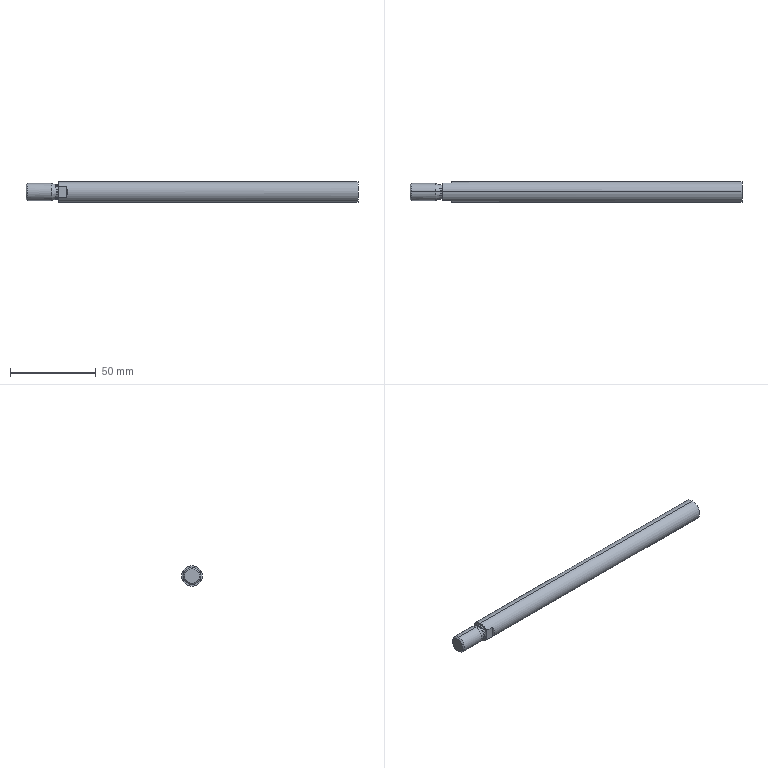Part | STEP file | HI_536288 ADN-150P0----(KS)_1-a_1_2 | 1 solid | 21 faces | box 193.7 x 12 x 12 mm | volume 21128 mm3 | plane 7 | cylinder 6 | spline 4 | cone 4 | commonest cylinder face diameters 8.2 x2 10 x2 12 x2